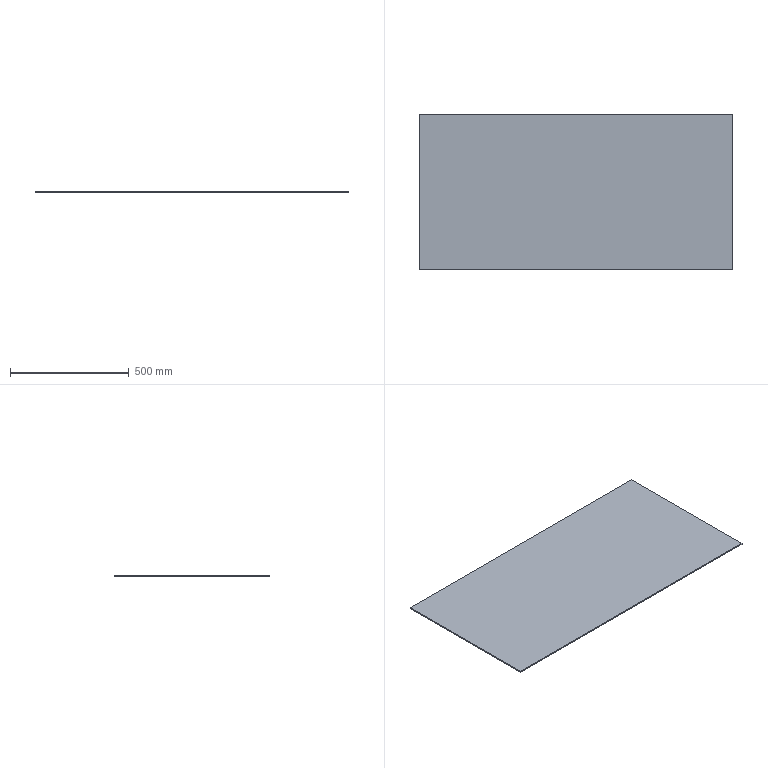Part | STEP file | 1 solid | 6 faces | box 1318 x 655 x 5 mm | volume 4316450 mm3 | plane 6
STEP:
#1=CARTESIAN_POINT('',(0.,0.,0.));
#2=DIRECTION('',(0.,0.,1.));
#3=DIRECTION('',(1.,0.,0.));
#4=AXIS2_PLACEMENT_3D('',#1,#2,#3);
#5=CARTESIAN_POINT('',(-659.,706.,0.));
#6=VERTEX_POINT('',#5);
#7=CARTESIAN_POINT('',(659.,706.,0.));
#8=VERTEX_POINT('',#7);
#9=CARTESIAN_POINT('',(659.,706.,0.));
#10=DIRECTION('',(1.,0.,0.));
#11=VECTOR('',#10,1.);
#12=LINE('',#9,#11);
#13=CARTESIAN_POINT('',(0.,0.,0.));
#14=DIRECTION('',(0.,0.,1.));
#15=DIRECTION('',(1.,0.,0.));
#16=AXIS2_PLACEMENT_3D('',#13,#14,#15);
#17=PLANE('',#16);
#18=CARTESIAN_POINT('',(659.,706.));
#19=DIRECTION('',(1.,0.));
#20=VECTOR('',#19,1.);
#21=LINE('',#18,#20);
#22=(GEOMETRIC_REPRESENTATION_CONTEXT(2)PARAMETRIC_REPRESENTATION_CONTEXT()REPRESENTATION_CONTEXT('',''));
#23=DEFINITIONAL_REPRESENTATION('',(#21),#22);
#24=PCURVE('',#17,#23);
#25=CARTESIAN_POINT('',(659.,706.,5.));
#26=DIRECTION('',(0.,-1.,0.));
#27=DIRECTION('',(0.,0.,-1.));
#28=AXIS2_PLACEMENT_3D('',#25,#26,#27);
#29=PLANE('',#28);
#30=CARTESIAN_POINT('',(5.,0.));
#31=DIRECTION('',(0.,1.));
#32=VECTOR('',#31,1.);
#33=LINE('',#30,#32);
#34=(GEOMETRIC_REPRESENTATION_CONTEXT(2)PARAMETRIC_REPRESENTATION_CONTEXT()REPRESENTATION_CONTEXT('',''));
#35=DEFINITIONAL_REPRESENTATION('',(#33),#34);
#36=PCURVE('',#29,#35);
#37=SURFACE_CURVE('',#12,(#24,#36),.PCURVE_S1.);
#38=EDGE_CURVE('',#6,#8,#37,.T.);
#39=ORIENTED_EDGE('',*,*,#38,.T.);
#40=CARTESIAN_POINT('',(659.,51.,0.));
#41=VERTEX_POINT('',#40);
#42=CARTESIAN_POINT('',(659.,51.,0.));
#43=DIRECTION('',(0.,-1.,0.));
#44=VECTOR('',#43,1.);
#45=LINE('',#42,#44);
#46=CARTESIAN_POINT('',(659.,51.));
#47=DIRECTION('',(0.,-1.));
#48=VECTOR('',#47,1.);
#49=LINE('',#46,#48);
#50=(GEOMETRIC_REPRESENTATION_CONTEXT(2)PARAMETRIC_REPRESENTATION_CONTEXT()REPRESENTATION_CONTEXT('',''));
#51=DEFINITIONAL_REPRESENTATION('',(#49),#50);
#52=PCURVE('',#17,#51);
#53=CARTESIAN_POINT('',(659.,51.,5.));
#54=DIRECTION('',(-1.,0.,0.));
#55=DIRECTION('',(0.,0.,1.));
#56=AXIS2_PLACEMENT_3D('',#53,#54,#55);
#57=PLANE('',#56);
#58=CARTESIAN_POINT('',(-5.,0.));
#59=DIRECTION('',(0.,-1.));
#60=VECTOR('',#59,1.);
#61=LINE('',#58,#60);
#62=(GEOMETRIC_REPRESENTATION_CONTEXT(2)PARAMETRIC_REPRESENTATION_CONTEXT()REPRESENTATION_CONTEXT('',''));
#63=DEFINITIONAL_REPRESENTATION('',(#61),#62);
#64=PCURVE('',#57,#63);
#65=SURFACE_CURVE('',#45,(#52,#64),.PCURVE_S1.);
#66=EDGE_CURVE('',#8,#41,#65,.T.);
#67=ORIENTED_EDGE('',*,*,#66,.T.);
#68=CARTESIAN_POINT('',(-659.,51.,0.));
#69=VERTEX_POINT('',#68);
#70=CARTESIAN_POINT('',(-659.,51.,0.));
#71=DIRECTION('',(-1.,0.,0.));
#72=VECTOR('',#71,1.);
#73=LINE('',#70,#72);
#74=CARTESIAN_POINT('',(-659.,51.));
#75=DIRECTION('',(-1.,0.));
#76=VECTOR('',#75,1.);
#77=LINE('',#74,#76);
#78=(GEOMETRIC_REPRESENTATION_CONTEXT(2)PARAMETRIC_REPRESENTATION_CONTEXT()REPRESENTATION_CONTEXT('',''));
#79=DEFINITIONAL_REPRESENTATION('',(#77),#78);
#80=PCURVE('',#17,#79);
#81=CARTESIAN_POINT('',(-659.,51.,5.));
#82=DIRECTION('',(0.,1.,0.));
#83=DIRECTION('',(1.,0.,0.));
#84=AXIS2_PLACEMENT_3D('',#81,#82,#83);
#85=PLANE('',#84);
#86=CARTESIAN_POINT('',(0.,5.));
#87=DIRECTION('',(-1.,0.));
#88=VECTOR('',#87,1.);
#89=LINE('',#86,#88);
#90=(GEOMETRIC_REPRESENTATION_CONTEXT(2)PARAMETRIC_REPRESENTATION_CONTEXT()REPRESENTATION_CONTEXT('',''));
#91=DEFINITIONAL_REPRESENTATION('',(#89),#90);
#92=PCURVE('',#85,#91);
#93=SURFACE_CURVE('',#73,(#80,#92),.PCURVE_S1.);
#94=EDGE_CURVE('',#41,#69,#93,.T.);
#95=ORIENTED_EDGE('',*,*,#94,.T.);
#96=CARTESIAN_POINT('',(-659.,706.,0.));
#97=DIRECTION('',(0.,1.,0.));
#98=VECTOR('',#97,1.);
#99=LINE('',#96,#98);
#100=CARTESIAN_POINT('',(-659.,706.));
#101=DIRECTION('',(0.,1.));
#102=VECTOR('',#101,1.);
#103=LINE('',#100,#102);
#104=(GEOMETRIC_REPRESENTATION_CONTEXT(2)PARAMETRIC_REPRESENTATION_CONTEXT()REPRESENTATION_CONTEXT('',''));
#105=DEFINITIONAL_REPRESENTATION('',(#103),#104);
#106=PCURVE('',#17,#105);
#107=CARTESIAN_POINT('',(-659.,706.,5.));
#108=DIRECTION('',(1.,0.,0.));
#109=DIRECTION('',(0.,1.,0.));
#110=AXIS2_PLACEMENT_3D('',#107,#108,#109);
#111=PLANE('',#110);
#112=CARTESIAN_POINT('',(0.,-5.));
#113=DIRECTION('',(1.,0.));
#114=VECTOR('',#113,1.);
#115=LINE('',#112,#114);
#116=(GEOMETRIC_REPRESENTATION_CONTEXT(2)PARAMETRIC_REPRESENTATION_CONTEXT()REPRESENTATION_CONTEXT('',''));
#117=DEFINITIONAL_REPRESENTATION('',(#115),#116);
#118=PCURVE('',#111,#117);
#119=SURFACE_CURVE('',#99,(#106,#118),.PCURVE_S1.);
#120=EDGE_CURVE('',#69,#6,#119,.T.);
#121=ORIENTED_EDGE('',*,*,#120,.T.);
#122=EDGE_LOOP('',(#39,#67,#95,#121));
#123=FACE_BOUND('',#122,.T.);
#124=ADVANCED_FACE('',(#123),#17,.F.);
#125=CARTESIAN_POINT('',(-659.,51.,5.));
#126=VERTEX_POINT('',#125);
#127=CARTESIAN_POINT('',(-659.,51.,5.));
#128=DIRECTION('',(0.,0.,1.));
#129=VECTOR('',#128,1.);
#130=LINE('',#127,#129);
#131=CARTESIAN_POINT('',(-655.,0.));
#132=DIRECTION('',(0.,1.));
#133=VECTOR('',#132,1.);
#134=LINE('',#131,#133);
#135=(GEOMETRIC_REPRESENTATION_CONTEXT(2)PARAMETRIC_REPRESENTATION_CONTEXT()REPRESENTATION_CONTEXT('',''));
#136=DEFINITIONAL_REPRESENTATION('',(#134),#135);
#137=PCURVE('',#111,#136);
#138=CARTESIAN_POINT('',(0.,0.));
#139=DIRECTION('',(0.,-1.));
#140=VECTOR('',#139,1.);
#141=LINE('',#138,#140);
#142=(GEOMETRIC_REPRESENTATION_CONTEXT(2)PARAMETRIC_REPRESENTATION_CONTEXT()REPRESENTATION_CONTEXT('',''));
#143=DEFINITIONAL_REPRESENTATION('',(#141),#142);
#144=PCURVE('',#85,#143);
#145=SURFACE_CURVE('',#130,(#137,#144),.PCURVE_S1.);
#146=EDGE_CURVE('',#69,#126,#145,.T.);
#147=ORIENTED_EDGE('',*,*,#146,.T.);
#148=CARTESIAN_POINT('',(-659.,706.,5.));
#149=VERTEX_POINT('',#148);
#150=CARTESIAN_POINT('',(-659.,0.,5.));
#151=DIRECTION('',(0.,-1.,0.));
#152=VECTOR('',#151,1.);
#153=LINE('',#150,#152);
#154=CARTESIAN_POINT('',(-706.,0.));
#155=DIRECTION('',(-1.,0.));
#156=VECTOR('',#155,1.);
#157=LINE('',#154,#156);
#158=(GEOMETRIC_REPRESENTATION_CONTEXT(2)PARAMETRIC_REPRESENTATION_CONTEXT()REPRESENTATION_CONTEXT('',''));
#159=DEFINITIONAL_REPRESENTATION('',(#157),#158);
#160=PCURVE('',#111,#159);
#161=CARTESIAN_POINT('',(0.,0.,5.));
#162=DIRECTION('',(0.,0.,1.));
#163=DIRECTION('',(1.,0.,0.));
#164=AXIS2_PLACEMENT_3D('',#161,#162,#163);
#165=PLANE('',#164);
#166=CARTESIAN_POINT('',(-659.,0.));
#167=DIRECTION('',(0.,-1.));
#168=VECTOR('',#167,1.);
#169=LINE('',#166,#168);
#170=(GEOMETRIC_REPRESENTATION_CONTEXT(2)PARAMETRIC_REPRESENTATION_CONTEXT()REPRESENTATION_CONTEXT('',''));
#171=DEFINITIONAL_REPRESENTATION('',(#169),#170);
#172=PCURVE('',#165,#171);
#173=SURFACE_CURVE('',#153,(#160,#172),.PCURVE_S1.);
#174=EDGE_CURVE('',#149,#126,#173,.T.);
#175=ORIENTED_EDGE('',*,*,#174,.F.);
#176=CARTESIAN_POINT('',(-659.,706.,5.));
#177=DIRECTION('',(0.,0.,-1.));
#178=VECTOR('',#177,1.);
#179=LINE('',#176,#178);
#180=CARTESIAN_POINT('',(0.,0.));
#181=DIRECTION('',(0.,-1.));
#182=VECTOR('',#181,1.);
#183=LINE('',#180,#182);
#184=(GEOMETRIC_REPRESENTATION_CONTEXT(2)PARAMETRIC_REPRESENTATION_CONTEXT()REPRESENTATION_CONTEXT('',''));
#185=DEFINITIONAL_REPRESENTATION('',(#183),#184);
#186=PCURVE('',#111,#185);
#187=CARTESIAN_POINT('',(0.,-1318.));
#188=DIRECTION('',(1.,0.));
#189=VECTOR('',#188,1.);
#190=LINE('',#187,#189);
#191=(GEOMETRIC_REPRESENTATION_CONTEXT(2)PARAMETRIC_REPRESENTATION_CONTEXT()REPRESENTATION_CONTEXT('',''));
#192=DEFINITIONAL_REPRESENTATION('',(#190),#191);
#193=PCURVE('',#29,#192);
#194=SURFACE_CURVE('',#179,(#186,#193),.PCURVE_S1.);
#195=EDGE_CURVE('',#149,#6,#194,.T.);
#196=ORIENTED_EDGE('',*,*,#195,.T.);
#197=ORIENTED_EDGE('',*,*,#120,.F.);
#198=EDGE_LOOP('',(#147,#175,#196,#197));
#199=FACE_BOUND('',#198,.T.);
#200=ADVANCED_FACE('',(#199),#111,.F.);
#201=CARTESIAN_POINT('',(659.,51.,5.));
#202=VERTEX_POINT('',#201);
#203=CARTESIAN_POINT('',(659.,51.,5.));
#204=DIRECTION('',(0.,0.,1.));
#205=VECTOR('',#204,1.);
#206=LINE('',#203,#205);
#207=CARTESIAN_POINT('',(1318.,0.));
#208=DIRECTION('',(0.,-1.));
#209=VECTOR('',#208,1.);
#210=LINE('',#207,#209);
#211=(GEOMETRIC_REPRESENTATION_CONTEXT(2)PARAMETRIC_REPRESENTATION_CONTEXT()REPRESENTATION_CONTEXT('',''));
#212=DEFINITIONAL_REPRESENTATION('',(#210),#211);
#213=PCURVE('',#85,#212);
#214=CARTESIAN_POINT('',(0.,0.));
#215=DIRECTION('',(1.,0.));
#216=VECTOR('',#215,1.);
#217=LINE('',#214,#216);
#218=(GEOMETRIC_REPRESENTATION_CONTEXT(2)PARAMETRIC_REPRESENTATION_CONTEXT()REPRESENTATION_CONTEXT('',''));
#219=DEFINITIONAL_REPRESENTATION('',(#217),#218);
#220=PCURVE('',#57,#219);
#221=SURFACE_CURVE('',#206,(#213,#220),.PCURVE_S1.);
#222=EDGE_CURVE('',#41,#202,#221,.T.);
#223=ORIENTED_EDGE('',*,*,#222,.T.);
#224=CARTESIAN_POINT('',(0.,51.,5.));
#225=DIRECTION('',(1.,0.,0.));
#226=VECTOR('',#225,1.);
#227=LINE('',#224,#226);
#228=CARTESIAN_POINT('',(659.,0.));
#229=DIRECTION('',(1.,0.));
#230=VECTOR('',#229,1.);
#231=LINE('',#228,#230);
#232=(GEOMETRIC_REPRESENTATION_CONTEXT(2)PARAMETRIC_REPRESENTATION_CONTEXT()REPRESENTATION_CONTEXT('',''));
#233=DEFINITIONAL_REPRESENTATION('',(#231),#232);
#234=PCURVE('',#85,#233);
#235=CARTESIAN_POINT('',(0.,51.));
#236=DIRECTION('',(1.,0.));
#237=VECTOR('',#236,1.);
#238=LINE('',#235,#237);
#239=(GEOMETRIC_REPRESENTATION_CONTEXT(2)PARAMETRIC_REPRESENTATION_CONTEXT()REPRESENTATION_CONTEXT('',''));
#240=DEFINITIONAL_REPRESENTATION('',(#238),#239);
#241=PCURVE('',#165,#240);
#242=SURFACE_CURVE('',#227,(#234,#241),.PCURVE_S1.);
#243=EDGE_CURVE('',#126,#202,#242,.T.);
#244=ORIENTED_EDGE('',*,*,#243,.F.);
#245=ORIENTED_EDGE('',*,*,#146,.F.);
#246=ORIENTED_EDGE('',*,*,#94,.F.);
#247=EDGE_LOOP('',(#223,#244,#245,#246));
#248=FACE_BOUND('',#247,.T.);
#249=ADVANCED_FACE('',(#248),#85,.F.);
#250=CARTESIAN_POINT('',(659.,706.,5.));
#251=VERTEX_POINT('',#250);
#252=CARTESIAN_POINT('',(659.,706.,5.));
#253=DIRECTION('',(0.,0.,1.));
#254=VECTOR('',#253,1.);
#255=LINE('',#252,#254);
#256=CARTESIAN_POINT('',(0.,655.));
#257=DIRECTION('',(1.,0.));
#258=VECTOR('',#257,1.);
#259=LINE('',#256,#258);
#260=(GEOMETRIC_REPRESENTATION_CONTEXT(2)PARAMETRIC_REPRESENTATION_CONTEXT()REPRESENTATION_CONTEXT('',''));
#261=DEFINITIONAL_REPRESENTATION('',(#259),#260);
#262=PCURVE('',#57,#261);
#263=CARTESIAN_POINT('',(0.,0.));
#264=DIRECTION('',(-1.,0.));
#265=VECTOR('',#264,1.);
#266=LINE('',#263,#265);
#267=(GEOMETRIC_REPRESENTATION_CONTEXT(2)PARAMETRIC_REPRESENTATION_CONTEXT()REPRESENTATION_CONTEXT('',''));
#268=DEFINITIONAL_REPRESENTATION('',(#266),#267);
#269=PCURVE('',#29,#268);
#270=SURFACE_CURVE('',#255,(#262,#269),.PCURVE_S1.);
#271=EDGE_CURVE('',#8,#251,#270,.T.);
#272=ORIENTED_EDGE('',*,*,#271,.T.);
#273=CARTESIAN_POINT('',(659.,0.,5.));
#274=DIRECTION('',(0.,1.,0.));
#275=VECTOR('',#274,1.);
#276=LINE('',#273,#275);
#277=CARTESIAN_POINT('',(0.,-51.));
#278=DIRECTION('',(0.,1.));
#279=VECTOR('',#278,1.);
#280=LINE('',#277,#279);
#281=(GEOMETRIC_REPRESENTATION_CONTEXT(2)PARAMETRIC_REPRESENTATION_CONTEXT()REPRESENTATION_CONTEXT('',''));
#282=DEFINITIONAL_REPRESENTATION('',(#280),#281);
#283=PCURVE('',#57,#282);
#284=CARTESIAN_POINT('',(659.,0.));
#285=DIRECTION('',(0.,1.));
#286=VECTOR('',#285,1.);
#287=LINE('',#284,#286);
#288=(GEOMETRIC_REPRESENTATION_CONTEXT(2)PARAMETRIC_REPRESENTATION_CONTEXT()REPRESENTATION_CONTEXT('',''));
#289=DEFINITIONAL_REPRESENTATION('',(#287),#288);
#290=PCURVE('',#165,#289);
#291=SURFACE_CURVE('',#276,(#283,#290),.PCURVE_S1.);
#292=EDGE_CURVE('',#202,#251,#291,.T.);
#293=ORIENTED_EDGE('',*,*,#292,.F.);
#294=ORIENTED_EDGE('',*,*,#222,.F.);
#295=ORIENTED_EDGE('',*,*,#66,.F.);
#296=EDGE_LOOP('',(#272,#293,#294,#295));
#297=FACE_BOUND('',#296,.T.);
#298=ADVANCED_FACE('',(#297),#57,.F.);
#299=ORIENTED_EDGE('',*,*,#195,.F.);
#300=CARTESIAN_POINT('',(0.,706.,5.));
#301=DIRECTION('',(-1.,0.,0.));
#302=VECTOR('',#301,1.);
#303=LINE('',#300,#302);
#304=CARTESIAN_POINT('',(0.,-659.));
#305=DIRECTION('',(0.,-1.));
#306=VECTOR('',#305,1.);
#307=LINE('',#304,#306);
#308=(GEOMETRIC_REPRESENTATION_CONTEXT(2)PARAMETRIC_REPRESENTATION_CONTEXT()REPRESENTATION_CONTEXT('',''));
#309=DEFINITIONAL_REPRESENTATION('',(#307),#308);
#310=PCURVE('',#29,#309);
#311=CARTESIAN_POINT('',(0.,706.));
#312=DIRECTION('',(-1.,0.));
#313=VECTOR('',#312,1.);
#314=LINE('',#311,#313);
#315=(GEOMETRIC_REPRESENTATION_CONTEXT(2)PARAMETRIC_REPRESENTATION_CONTEXT()REPRESENTATION_CONTEXT('',''));
#316=DEFINITIONAL_REPRESENTATION('',(#314),#315);
#317=PCURVE('',#165,#316);
#318=SURFACE_CURVE('',#303,(#310,#317),.PCURVE_S1.);
#319=EDGE_CURVE('',#251,#149,#318,.T.);
#320=ORIENTED_EDGE('',*,*,#319,.F.);
#321=ORIENTED_EDGE('',*,*,#271,.F.);
#322=ORIENTED_EDGE('',*,*,#38,.F.);
#323=EDGE_LOOP('',(#299,#320,#321,#322));
#324=FACE_BOUND('',#323,.T.);
#325=ADVANCED_FACE('',(#324),#29,.F.);
#326=ORIENTED_EDGE('',*,*,#292,.T.);
#327=ORIENTED_EDGE('',*,*,#319,.T.);
#328=ORIENTED_EDGE('',*,*,#174,.T.);
#329=ORIENTED_EDGE('',*,*,#243,.T.);
#330=EDGE_LOOP('',(#326,#327,#328,#329));
#331=FACE_BOUND('',#330,.T.);
#332=ADVANCED_FACE('',(#331),#165,.T.);
#333=CLOSED_SHELL('',(#124,#200,#249,#298,#325,#332));
#334=MANIFOLD_SOLID_BREP('',#333);
#335=(LENGTH_UNIT()NAMED_UNIT(*)SI_UNIT(.MILLI.,.METRE.));
#336=UNCERTAINTY_MEASURE_WITH_UNIT(LENGTH_MEASURE(0.0000001),#335,'','');
#337=(NAMED_UNIT(*)PLANE_ANGLE_UNIT()SI_UNIT($,.RADIAN.));
#338=(NAMED_UNIT(*)SI_UNIT($,.STERADIAN.)SOLID_ANGLE_UNIT());
#339=(GEOMETRIC_REPRESENTATION_CONTEXT(3)GLOBAL_UNCERTAINTY_ASSIGNED_CONTEXT((#336))GLOBAL_UNIT_ASSIGNED_CONTEXT((#335,#337,#338))REPRESENTATION_CONTEXT('',''));
#340=ADVANCED_BREP_SHAPE_REPRESENTATION('',(#4,#334),#339);